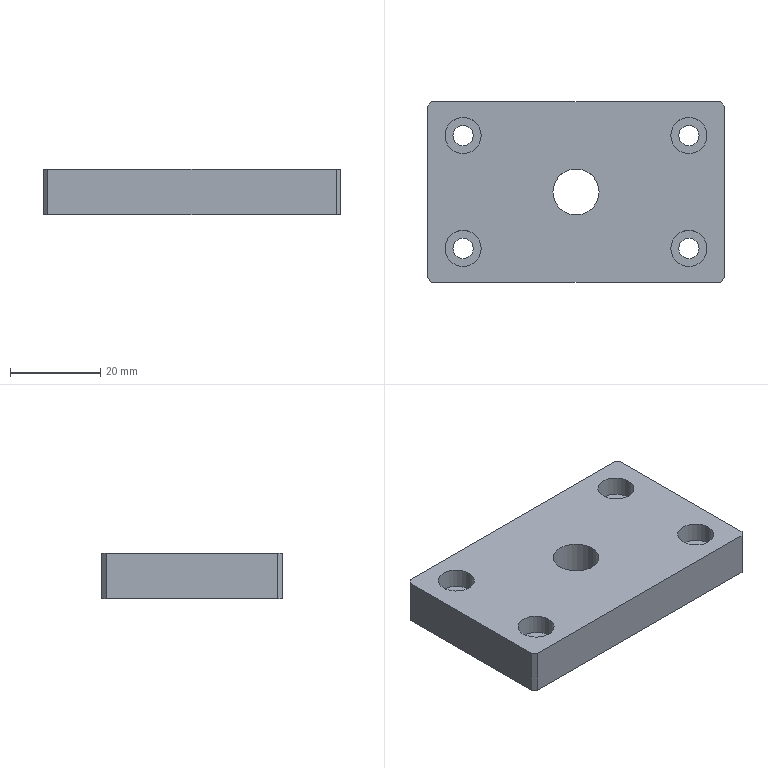Part | STEP file | PN_0035 | 1 solid | 32 faces | box 66 x 40 x 10 mm | volume 24322 mm3 | cylinder 18 | plane 14 | commonest cylinder face diameters 4.5 x8 8 x8 10.2 x2